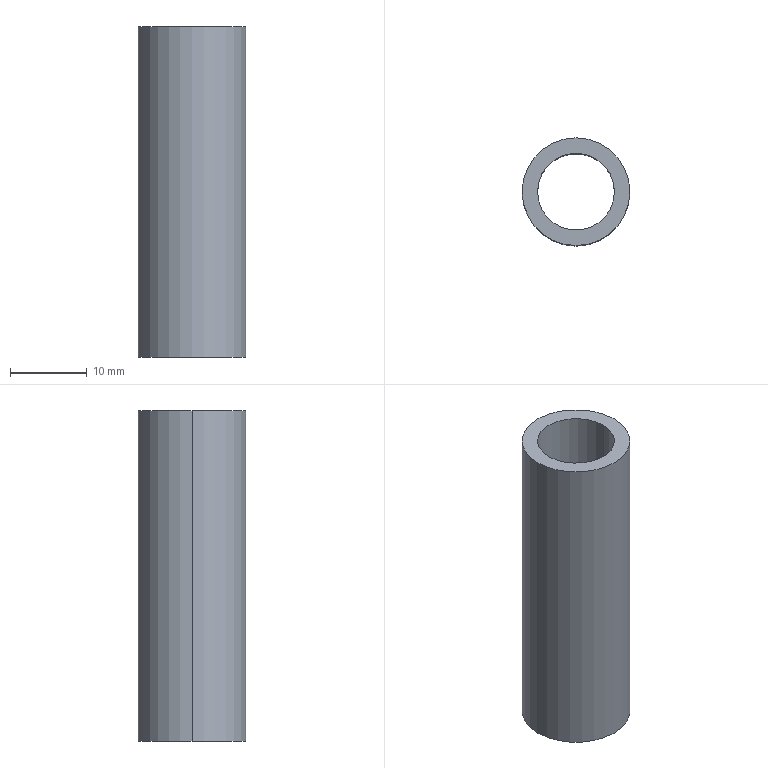Part | SolidWorks | features Extrusion 1 | 1 solid | 6 faces | box 14 x 14 x 43 mm | volume 3242 mm3 | cylinder 4 | plane 2 | commonest cylinder face diameters 10 x2 14 x2
STEP:
#1=CARTESIAN_POINT('',(-5.,0.,43.));
#2=VERTEX_POINT('',#1);
#3=CARTESIAN_POINT('',(5.,0.,43.));
#4=VERTEX_POINT('',#3);
#5=CARTESIAN_POINT('',(0.,0.,43.));
#6=DIRECTION('',(0.,0.,1.));
#7=DIRECTION('',(1.,0.,0.));
#8=AXIS2_PLACEMENT_3D('',#5,#6,#7);
#9=CIRCLE('',#8,5.);
#10=EDGE_CURVE('',#2,#4,#9,.T.);
#11=ORIENTED_EDGE('',*,*,#10,.T.);
#12=CARTESIAN_POINT('',(5.,0.,0.));
#13=VERTEX_POINT('',#12);
#14=CARTESIAN_POINT('',(5.,0.,43.));
#15=DIRECTION('',(0.,0.,-1.));
#16=VECTOR('',#15,1000.);
#17=LINE('',#14,#16);
#18=EDGE_CURVE('',#4,#13,#17,.T.);
#19=ORIENTED_EDGE('',*,*,#18,.T.);
#20=CARTESIAN_POINT('',(-5.,0.,0.));
#21=VERTEX_POINT('',#20);
#22=CARTESIAN_POINT('',(0.,0.,0.));
#23=DIRECTION('',(0.,0.,1.));
#24=DIRECTION('',(1.,0.,0.));
#25=AXIS2_PLACEMENT_3D('',#22,#23,#24);
#26=CIRCLE('',#25,5.);
#27=EDGE_CURVE('',#21,#13,#26,.T.);
#28=ORIENTED_EDGE('',*,*,#27,.F.);
#29=CARTESIAN_POINT('',(-5.,0.,43.));
#30=DIRECTION('',(0.,0.,-1.));
#31=VECTOR('',#30,1000.);
#32=LINE('',#29,#31);
#33=EDGE_CURVE('',#2,#21,#32,.T.);
#34=ORIENTED_EDGE('',*,*,#33,.F.);
#35=EDGE_LOOP('',(#11,#19,#28,#34));
#36=FACE_OUTER_BOUND('',#35,.T.);
#37=CARTESIAN_POINT('',(0.,0.,43.));
#38=DIRECTION('',(0.,0.,-1.));
#39=DIRECTION('',(-1.,0.,0.));
#40=AXIS2_PLACEMENT_3D('',#37,#38,#39);
#41=CYLINDRICAL_SURFACE('',#40,5.);
#42=ADVANCED_FACE('',(#36),#41,.F.);
#43=CARTESIAN_POINT('',(7.,0.,43.));
#44=VERTEX_POINT('',#43);
#45=CARTESIAN_POINT('',(-7.,0.,43.));
#46=VERTEX_POINT('',#45);
#47=CARTESIAN_POINT('',(0.,0.,43.));
#48=DIRECTION('',(0.,0.,1.));
#49=DIRECTION('',(1.,0.,0.));
#50=AXIS2_PLACEMENT_3D('',#47,#48,#49);
#51=CIRCLE('',#50,7.);
#52=EDGE_CURVE('',#44,#46,#51,.T.);
#53=ORIENTED_EDGE('',*,*,#52,.F.);
#54=CARTESIAN_POINT('',(7.,0.,0.));
#55=VERTEX_POINT('',#54);
#56=CARTESIAN_POINT('',(7.,0.,43.));
#57=DIRECTION('',(0.,0.,-1.));
#58=VECTOR('',#57,1000.);
#59=LINE('',#56,#58);
#60=EDGE_CURVE('',#44,#55,#59,.T.);
#61=ORIENTED_EDGE('',*,*,#60,.T.);
#62=CARTESIAN_POINT('',(-7.,0.,0.));
#63=VERTEX_POINT('',#62);
#64=CARTESIAN_POINT('',(0.,0.,0.));
#65=DIRECTION('',(0.,0.,1.));
#66=DIRECTION('',(1.,0.,0.));
#67=AXIS2_PLACEMENT_3D('',#64,#65,#66);
#68=CIRCLE('',#67,7.);
#69=EDGE_CURVE('',#55,#63,#68,.T.);
#70=ORIENTED_EDGE('',*,*,#69,.T.);
#71=CARTESIAN_POINT('',(-7.,0.,43.));
#72=DIRECTION('',(0.,0.,-1.));
#73=VECTOR('',#72,1000.);
#74=LINE('',#71,#73);
#75=EDGE_CURVE('',#46,#63,#74,.T.);
#76=ORIENTED_EDGE('',*,*,#75,.F.);
#77=EDGE_LOOP('',(#53,#61,#70,#76));
#78=FACE_OUTER_BOUND('',#77,.T.);
#79=CARTESIAN_POINT('',(0.,0.,43.));
#80=DIRECTION('',(0.,0.,-1.));
#81=DIRECTION('',(-1.,0.,0.));
#82=AXIS2_PLACEMENT_3D('',#79,#80,#81);
#83=CYLINDRICAL_SURFACE('',#82,7.);
#84=ADVANCED_FACE('',(#78),#83,.T.);
#85=CARTESIAN_POINT('',(0.,0.,43.));
#86=DIRECTION('',(0.,0.,1.));
#87=DIRECTION('',(1.,0.,0.));
#88=AXIS2_PLACEMENT_3D('',#85,#86,#87);
#89=CIRCLE('',#88,7.);
#90=EDGE_CURVE('',#46,#44,#89,.T.);
#91=ORIENTED_EDGE('',*,*,#90,.T.);
#92=ORIENTED_EDGE('',*,*,#52,.T.);
#93=EDGE_LOOP('',(#91,#92));
#94=FACE_OUTER_BOUND('',#93,.T.);
#95=ORIENTED_EDGE('',*,*,#10,.F.);
#96=CARTESIAN_POINT('',(0.,0.,43.));
#97=DIRECTION('',(0.,0.,1.));
#98=DIRECTION('',(1.,0.,0.));
#99=AXIS2_PLACEMENT_3D('',#96,#97,#98);
#100=CIRCLE('',#99,5.);
#101=EDGE_CURVE('',#4,#2,#100,.T.);
#102=ORIENTED_EDGE('',*,*,#101,.F.);
#103=EDGE_LOOP('',(#95,#102));
#104=FACE_BOUND('',#103,.T.);
#105=CARTESIAN_POINT('',(0.,0.,43.));
#106=DIRECTION('',(0.,0.,1.));
#107=DIRECTION('',(1.,0.,0.));
#108=AXIS2_PLACEMENT_3D('',#105,#106,#107);
#109=PLANE('',#108);
#110=ADVANCED_FACE('',(#94,#104),#109,.T.);
#111=CARTESIAN_POINT('',(0.,0.,0.));
#112=DIRECTION('',(0.,0.,1.));
#113=DIRECTION('',(1.,0.,0.));
#114=AXIS2_PLACEMENT_3D('',#111,#112,#113);
#115=CIRCLE('',#114,7.);
#116=EDGE_CURVE('',#63,#55,#115,.T.);
#117=ORIENTED_EDGE('',*,*,#116,.F.);
#118=ORIENTED_EDGE('',*,*,#69,.F.);
#119=EDGE_LOOP('',(#117,#118));
#120=FACE_OUTER_BOUND('',#119,.T.);
#121=ORIENTED_EDGE('',*,*,#27,.T.);
#122=CARTESIAN_POINT('',(0.,0.,0.));
#123=DIRECTION('',(0.,0.,1.));
#124=DIRECTION('',(1.,0.,0.));
#125=AXIS2_PLACEMENT_3D('',#122,#123,#124);
#126=CIRCLE('',#125,5.);
#127=EDGE_CURVE('',#13,#21,#126,.T.);
#128=ORIENTED_EDGE('',*,*,#127,.T.);
#129=EDGE_LOOP('',(#121,#128));
#130=FACE_BOUND('',#129,.T.);
#131=CARTESIAN_POINT('',(0.,0.,0.));
#132=DIRECTION('',(0.,0.,1.));
#133=DIRECTION('',(1.,0.,0.));
#134=AXIS2_PLACEMENT_3D('',#131,#132,#133);
#135=PLANE('',#134);
#136=ADVANCED_FACE('',(#120,#130),#135,.F.);
#137=ORIENTED_EDGE('',*,*,#60,.F.);
#138=ORIENTED_EDGE('',*,*,#90,.F.);
#139=ORIENTED_EDGE('',*,*,#75,.T.);
#140=ORIENTED_EDGE('',*,*,#116,.T.);
#141=EDGE_LOOP('',(#137,#138,#139,#140));
#142=FACE_OUTER_BOUND('',#141,.T.);
#143=CARTESIAN_POINT('',(0.,0.,43.));
#144=DIRECTION('',(0.,0.,-1.));
#145=DIRECTION('',(-1.,0.,0.));
#146=AXIS2_PLACEMENT_3D('',#143,#144,#145);
#147=CYLINDRICAL_SURFACE('',#146,7.);
#148=ADVANCED_FACE('',(#142),#147,.T.);
#149=ORIENTED_EDGE('',*,*,#18,.F.);
#150=ORIENTED_EDGE('',*,*,#101,.T.);
#151=ORIENTED_EDGE('',*,*,#33,.T.);
#152=ORIENTED_EDGE('',*,*,#127,.F.);
#153=EDGE_LOOP('',(#149,#150,#151,#152));
#154=FACE_OUTER_BOUND('',#153,.T.);
#155=CARTESIAN_POINT('',(0.,0.,43.));
#156=DIRECTION('',(0.,0.,-1.));
#157=DIRECTION('',(-1.,0.,0.));
#158=AXIS2_PLACEMENT_3D('',#155,#156,#157);
#159=CYLINDRICAL_SURFACE('',#158,5.);
#160=ADVANCED_FACE('',(#154),#159,.F.);
#161=CLOSED_SHELL('',(#42,#84,#110,#136,#148,#160));
#162=MANIFOLD_SOLID_BREP('',#161);
#163=CARTESIAN_POINT('',(0.,0.,0.));
#164=DIRECTION('',(0.,0.,1.));
#165=DIRECTION('',(1.,0.,0.));
#166=AXIS2_PLACEMENT_3D('',#163,#164,#165);
#167=(LENGTH_UNIT()NAMED_UNIT(*)SI_UNIT(.MILLI.,.METRE.));
#168=UNCERTAINTY_MEASURE_WITH_UNIT(LENGTH_MEASURE(0.00001),#167,'','');
#169=(NAMED_UNIT(*)PLANE_ANGLE_UNIT()SI_UNIT($,.RADIAN.));
#170=(NAMED_UNIT(*)SI_UNIT($,.STERADIAN.)SOLID_ANGLE_UNIT());
#171=(GEOMETRIC_REPRESENTATION_CONTEXT(3)GLOBAL_UNCERTAINTY_ASSIGNED_CONTEXT((#168))GLOBAL_UNIT_ASSIGNED_CONTEXT((#167,#169,#170))REPRESENTATION_CONTEXT('',''));
#172=ADVANCED_BREP_SHAPE_REPRESENTATION('',(#162,#166),#171);